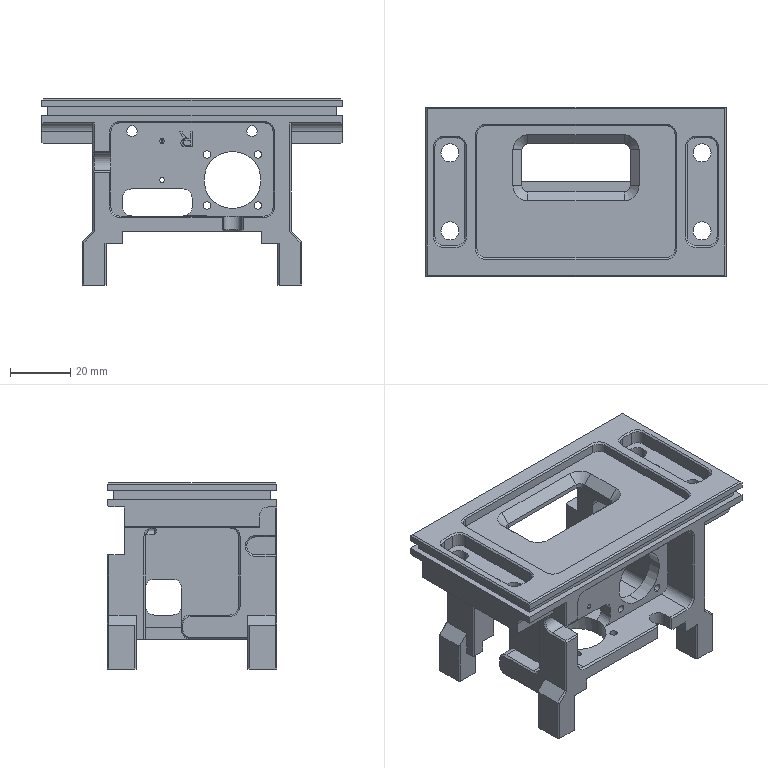CAM job | Mastercam | 3-axis milling, drilling | part box 100 x 56.5 x 62 mm | stock box 110 x 56.5 x 80 mm
Tools:
tool_number,name,type,diameter_mm,corner_radius_mm,flutes,flute_length_mm,overall_length_mm,shoulder_length_mm,holder_diameter_mm,length_offset,diameter_offset,default_rpm,default_feed_mm_min,default_plunge_mm_min,coolant
2,2 Flat End Mill,end mill,2,0,4,25,75,25,50,2,2,5000,600,600,COOL_OFF
2,2 Flat End Mill,end mill,2,0,4,25,75,25,50,2,2,5000,600,600,COOL_OFF
3,3 Flat End Mill,end mill,3,0,4,25,75,25,50,3,3,3333,399.96,600,COOL_OFF
3,3 Flat End Mill,end mill,3,0,4,25,75,25,50,3,3,3333,399.96,600,COOL_OFF
4,4 Flat End Mill,end mill,4,0,4,25,75,25,50,4,4,2500,300,600,COOL_OFF
4,4 Flat End Mill,end mill,4,0,4,25,75,25,50,4,4,2500,300,600,COOL_OFF
5,4 Chamfer Mill,chamfer mill,4,0,4,25,75,30,50,5,5,6250,750,600,COOL_OFF
5,4 Chamfer Mill,chamfer mill,4,0,4,25,75,30,50,5,5,6250,750,600,COOL_OFF
5,6 Flat End Mill,end mill,6,0,4,25,75,25,50,5,5,1667,200.04,600,COOL_OFF
6,6 Flat End Mill,end mill,6,0,4,25,75,25,50,6,6,1667,200.04,600,COOL_OFF
6,6 Flat End Mill,end mill,6,0,4,25,75,25,50,6,6,1667,200.04,600,COOL_OFF
11,12 Flat End Mill,end mill,12,0,4,25,75,25,50,11,11,8000,4000,600,COOL_OFF
11,12 Flat End Mill,end mill,12,0,4,25,75,25,50,11,11,8000,4000,600,COOL_OFF
12,12 Flat End Mill,end mill,12,0,4,25,75,25,50,12,12,833,99.96,600,COOL_OFF
12,12 Flat End Mill,end mill,12,0,4,25,75,25,50,12,12,833,99.96,600,COOL_OFF
13,16 Flat End Mill,end mill,16,0,4,25,75,25,50,13,13,5000,3000,600,COOL_OFF
13,Copy 16 Flat End Mill,end mill,16,0,4,25,75,25,50,13,13,5000,3000,600,COOL_OFF
13,16 Flat End Mill,end mill,16,0,4,25,75,25,50,13,13,5000,3000,600,COOL_OFF
14,6 Flat End Mill,end mill,6,0,4,25,75,25,50,14,14,5000,2000,600,COOL_OFF
14,Copy 6 Flat End Mill,end mill,6,0,4,25,75,25,50,14,14,5000,2000,600,COOL_OFF
15,4 Flat End Mill,end mill,4,0,4,25,75,25,50,15,15,6500,2000,600,COOL_OFF
15,Copy 4 Flat End Mill,end mill,4,0,4,25,75,25,50,15,15,6500,2000,600,COOL_OFF
16,16 Flat End Mill,end mill,16,0,4,25,75,25,50,16,16,625,75,600,COOL_OFF
16,16 Flat End Mill,end mill,16,0,4,25,75,25,50,16,16,5000,1000,600,COOL_OFF
17,14 Chamfer Mill,chamfer mill,14,0,4,25,75,30,50,17,17,1786,214.32,600,COOL_OFF
17,14 Chamfer Mill,chamfer mill,14,0,4,25,75,30,50,17,17,1786,214.32,600,COOL_OFF
18,6 Flat End Mill,end mill,6,0,4,25,75,25,50,18,18,1667,200.04,600,COOL_OFF
18,Copy 6 Flat End Mill,end mill,6,0,4,25,75,25,50,18,18,1667,200.04,600,COOL_OFF
20,63 Flat End Mill,end mill,63,0,4,25,75,25,50,20,20,4000,1000,600,COOL_OFF
20,63 Flat End Mill,end mill,63,0,4,25,75,25,50,20,20,159,19.08,600,COOL_OFF
Operations:
seq,operation,operation_type,tool_number,tool_name,tool_diameter_mm,spindle_rpm,feed_mm_min,plunge_mm_min,retract_mm_min,cycle_time_s,wcs,posted,nc_file
1,Facing - [WCS: Plane] - [Tplane: Plane],Facing,20,63 Flat End Mill,63,4000,1000,600,1200,24.268,Plane,yes,1.nc
2,2D High Speed (2D Dynamic Mill) - [WCS: Plane] - [Tplane: Plane],HighSpeed2D,13,16 Flat End Mill,16,5500,3000,600,1200,372.445,Plane,yes,1.nc
3,Contour (Ramp) - [WCS: Plane] - [Tplane: Plane],Contour,13,16 Flat End Mill,16,5500,1500,600,1200,67.168,Plane,yes,1.nc
4,Contour (2D) - [WCS: Plane] - [Tplane: Plane],Contour,16,16 Flat End Mill,16,5500,1000,600,1200,51.918,Plane,yes,1.nc
5,Contour (Remachining) - [WCS: Plane] - [Tplane: Plane],Contour,6,6 Flat End Mill,6,7000,3000,600,1200,34.787,Plane,yes,1.nc
6,Contour (2D) - [WCS: Plane] - [Tplane: Plane],Contour,6,6 Flat End Mill,6,7000,1000,600,1200,37.219,Plane,yes,1.nc
7,2D High Speed (2D Area Mill) - [WCS: Plane] - [Tplane: Plane],HighSpeed2D,6,6 Flat End Mill,6,7000,1000,600,1200,26.955,Plane,yes,1.nc
8,Contour (Ramp) - [WCS: Plane] - [Tplane: Plane],Contour,6,6 Flat End Mill,6,7000,1500,600,1200,26.435,Plane,yes,1.nc
9,Contour (2D) - [WCS: Plane] - [Tplane: Plane],Contour,6,6 Flat End Mill,6,7000,1000,600,1200,8.281,Plane,yes,1.nc
10,Contour (Ramp) - [WCS: Plane] - [Tplane: Plane],Contour,6,6 Flat End Mill,6,7000,1500,600,1200,17.872,Plane,yes,1.nc
11,Contour (2D) - [WCS: Plane] - [Tplane: Plane],Contour,6,6 Flat End Mill,6,7000,1000,600,1200,8.664,Plane,yes,1.nc
12,Contour (Ramp) - [WCS: Plane] - [Tplane: Plane],Contour,2,2 Flat End Mill,2,7000,3000,600,1200,42.583,Plane,yes,1.nc
13,Contour (2D) - [WCS: Plane] - [Tplane: Plane],Contour,2,2 Flat End Mill,2,7000,800,600,1200,16.213,Plane,yes,1.nc
14,Contour (2D chamfer) - [WCS: Plane] - [Tplane: Plane],Contour,5,6 Flat End Mill,6,7000,1200,600,1200,16.866,Plane,yes,1.nc
15,Contour (2D chamfer) - [WCS: Plane] - [Tplane: Plane],Contour,5,6 Flat End Mill,6,7000,1200,600,1200,8.527,Plane,yes,1.nc
16,Contour (2D chamfer) - [WCS: Plane] - [Tplane: Plane],Contour,5,6 Flat End Mill,6,7000,1200,600,1200,18.288,Plane,yes,1.nc
17,Drill/Counterbore - [WCS: Plane] - [Tplane: Plane],Drill,5,6 Flat End Mill,6,6500,200,600,1200,6.526,Plane,yes,1.nc
18,Facing - [WCS: Plane-1] - [Tplane: Plane-1],Facing,20,63 Flat End Mill,63,4000,2000,600,1200,235.558,Plane-1,yes,1.nc
19,Contour (Ramp) - [WCS: Plane-1] - [Tplane: Plane-1],Contour,11,12 Flat End Mill,12,8000,4000,600,1200,34.159,Plane-1,yes,1.nc
20,Contour (2D) - [WCS: Plane-1] - [Tplane: Plane-1],Contour,12,12 Flat End Mill,12,8000,1000,600,1200,15.085,Plane-1,yes,1.nc
21,2D High Speed (2D Area Mill) - [WCS: Plane-1] - [Tplane: Plane-1],HighSpeed2D,11,12 Flat End Mill,12,8000,4000,600,1200,192.884,Plane-1,yes,1.nc
22,Contour (2D) - [WCS: Plane-1] - [Tplane: Plane-1],Contour,12,12 Flat End Mill,12,8000,1000,600,1200,18.911,Plane-1,yes,1.nc
23,Contour (Ramp) - [WCS: Plane-1] - [Tplane: Plane-1],Contour,11,12 Flat End Mill,12,8000,2000,600,1200,44.183,Plane-1,yes,1.nc
24,Contour (2D) - [WCS: Plane-1] - [Tplane: Plane-1],Contour,12,12 Flat End Mill,12,8000,1000,600,1200,7.27,Plane-1,yes,1.nc
25,Contour (Ramp) - [WCS: Plane-1] - [Tplane: Plane-1],Contour,11,12 Flat End Mill,12,8000,2000,600,1200,42.433,Plane-1,yes,1.nc
26,Contour (Remachining) - [WCS: Plane-1] - [Tplane: Plane-1],Contour,14,Copy 6 Flat End Mill,6,5000,3000,600,1200,35.027,Plane-1,yes,1.nc
27,2D High Speed (2D Area Mill) - [WCS: Plane-1] - [Tplane: Plane-1],HighSpeed2D,14,Copy 6 Flat End Mill,6,5000,800,600,1200,32.203,Plane-1,yes,1.nc
28,Contour (2D) - [WCS: Plane-1] - [Tplane: Plane-1],Contour,14,Copy 6 Flat End Mill,6,5000,800,600,1200,37.956,Plane-1,yes,1.nc
29,Contour (Remachining) - [WCS: Plane-1] - [Tplane: Plane-1],Contour,15,Copy 4 Flat End Mill,4,5500,2000,600,1200,46.379,Plane-1,yes,1.nc
30,Contour (Remachining) - [WCS: Plane-1] - [Tplane: Plane-1],Contour,15,Copy 4 Flat End Mill,4,5500,800,600,1200,20.427,Plane-1,yes,1.nc
31,Contour (Ramp) - [WCS: Plane-1] - [Tplane: Plane-1],Contour,2,2 Flat End Mill,2,6500,2000,600,1200,94.193,Plane-1,yes,1.nc
32,Contour (2D) - [WCS: Plane-1] - [Tplane: Plane-1],Contour,2,2 Flat End Mill,2,6500,1000,600,1200,13.093,Plane-1,yes,1.nc
33,Drill/Counterbore - [WCS: Plane-1] - [Tplane: Plane-1],Drill,5,6 Flat End Mill,6,6500,200,600,1200,1.512,Plane-1,yes,1.nc
34,Contour (2D chamfer) - [WCS: Plane-1] - [Tplane: Plane-1],Contour,5,6 Flat End Mill,6,6500,1000,600,1200,6.992,Plane-1,yes,1.nc
35,Contour (2D chamfer) - [WCS: Plane-1] - [Tplane: Plane-1],Contour,5,6 Flat End Mill,6,6500,1000,600,1200,6.846,Plane-1,yes,1.nc
36,Contour (2D chamfer) - [WCS: Plane-1] - [Tplane: Plane-1],Contour,5,6 Flat End Mill,6,6500,1000,600,1200,10.432,Plane-1,yes,1.nc
37,Contour (2D chamfer) - [WCS: Plane-1] - [Tplane: Plane-1],Contour,5,6 Flat End Mill,6,6500,1000,600,1200,11.317,Plane-1,yes,1.nc
38,Contour (2D chamfer) - [WCS: Plane-1] - [Tplane: Plane-1],Contour,5,6 Flat End Mill,6,6500,1000,600,1200,20.167,Plane-1,yes,1.nc
39,2D High Speed (2D Area Mill) - [WCS: Plane-2] - [Tplane: Plane-2],HighSpeed2D,11,12 Flat End Mill,12,8000,4000,600,1200,39.518,Plane-2,yes,1.nc
40,Contour (Ramp) - [WCS: Plane-2] - [Tplane: Plane-2],Contour,11,12 Flat End Mill,12,8000,2000,600,1200,14.081,Plane-2,yes,1.nc
41,Contour (Ramp) - [WCS: Plane-2] - [Tplane: Plane-2],Contour,6,6 Flat End Mill,6,6500,3000,600,1200,36.258,Plane-2,yes,1.nc
42,Contour (2D) - [WCS: Plane-2] - [Tplane: Plane-2],Contour,6,6 Flat End Mill,6,6500,1000,600,1200,26.145,Plane-2,yes,1.nc
43,Contour (Remachining) - [WCS: Plane-2] - [Tplane: Plane-2],Contour,6,6 Flat End Mill,6,6500,3000,600,1200,8.854,Plane-2,yes,1.nc
44,2D High Speed (2D Area Mill) - [WCS: Plane-2] - [Tplane: Plane-2],HighSpeed2D,6,6 Flat End Mill,6,6500,1000,600,1200,68.692,Plane-2,yes,1.nc
45,Contour (2D) - [WCS: Plane-2] - [Tplane: Plane-2],Contour,6,6 Flat End Mill,6,6500,1000,600,1200,36.067,Plane-2,yes,1.nc
46,Contour (Remachining) - [WCS: Plane-2] - [Tplane: Plane-2],Contour,3,3 Flat End Mill,3,6500,2000,600,1200,29.382,Plane-2,yes,1.nc
47,Contour (2D) - [WCS: Plane-2] - [Tplane: Plane-2],Contour,3,3 Flat End Mill,3,6500,1000,600,1200,11.957,Plane-2,yes,1.nc
48,Drill/Counterbore - [WCS: Plane-2] - [Tplane: Plane-2],Drill,5,6 Flat End Mill,6,6500,200,600,1200,2.994,Plane-2,yes,1.nc
49,Contour (2D chamfer) - [WCS: Plane-2] - [Tplane: Plane-2],Contour,5,6 Flat End Mill,6,6500,1000,600,1200,43.634,Plane-2,yes,1.nc
50,Contour (2D chamfer) - [WCS: Plane-2] - [Tplane: Plane-2],Contour,17,14 Chamfer Mill,14,6500,1000,600,1200,26.895,Plane-2,yes,1.nc
51,Contour (Ramp) - [WCS: Plane-2] - [Tplane: Plane-2],Contour,4,4 Flat End Mill,4,7000,2000,600,1200,13.401,Plane-2,yes,1.nc
52,Contour (Ramp) - [WCS: Plane-2] - [Tplane: Plane-2],Contour,4,4 Flat End Mill,4,7000,500,600,1200,10.581,Plane-2,yes,1.nc
53,Contour (2D) - [WCS: Plane-3] - [Tplane: Plane-3],Contour,13,16 Flat End Mill,16,5500,3000,600,1200,145.31,Plane-3,yes,1.nc
54,Contour (Ramp) - [WCS: Plane-3] - [Tplane: Plane-3],Contour,13,16 Flat End Mill,16,5500,3000,600,1200,16.646,Plane-3,yes,1.nc
55,Contour (Ramp) - [WCS: Plane-3] - [Tplane: Plane-3],Contour,13,16 Flat End Mill,16,5500,3000,600,1200,18.755,Plane-3,yes,1.nc
56,Contour (Ramp) - [WCS: Plane-3] - [Tplane: Plane-3],Contour,13,16 Flat End Mill,16,5500,2000,600,1200,13.738,Plane-3,yes,1.nc
57,Facing - [WCS: Plane-3] - [Tplane: Plane-3],Facing,16,16 Flat End Mill,16,5500,1000,600,1200,4.49,Plane-3,yes,1.nc
58,Contour (2D) - [WCS: Plane-3] - [Tplane: Plane-3],Contour,16,16 Flat End Mill,16,5500,1000,600,1200,9.961,Plane-3,yes,1.nc
59,Contour (2D) - [WCS: Plane-3] - [Tplane: Plane-3],Contour,16,16 Flat End Mill,16,5500,1000,600,1200,11.19,Plane-3,yes,1.nc
60,Contour (Ramp) - [WCS: Plane-3] - [Tplane: Plane-3],Contour,6,6 Flat End Mill,6,6500,3000,600,1200,15.861,Plane-3,yes,1.nc
61,Contour (2D) - [WCS: Plane-3] - [Tplane: Plane-3],Contour,6,6 Flat End Mill,6,6500,1000,600,1200,6.801,Plane-3,yes,1.nc
62,Contour (Remachining) - [WCS: Plane-3] - [Tplane: Plane-3],Contour,6,6 Flat End Mill,6,6500,3000,600,1200,15.343,Plane-3,yes,1.nc
63,Contour (2D) - [WCS: Plane-3] - [Tplane: Plane-3],Contour,6,6 Flat End Mill,6,6500,1000,600,1200,6.417,Plane-3,yes,1.nc
64,2D High Speed (2D Area Mill) - [WCS: Plane-3] - [Tplane: Plane-3],HighSpeed2D,6,6 Flat End Mill,6,6500,1000,600,1200,20.992,Plane-3,yes,1.nc
65,Contour (Ramp) - [WCS: Plane-3] - [Tplane: Plane-3],Contour,6,6 Flat End Mill,6,6500,2000,600,1200,30.854,Plane-3,yes,1.nc
66,Contour (2D) - [WCS: Plane-3] - [Tplane: Plane-3],Contour,6,6 Flat End Mill,6,6500,1000,600,1200,4.121,Plane-3,yes,1.nc
67,Contour (2D chamfer) - [WCS: Plane-3] - [Tplane: Plane-3],Contour,17,14 Chamfer Mill,14,6500,1000,600,1200,21.117,Plane-3,yes,1.nc
68,Contour (Ramp) - [WCS: Plane-3] - [Tplane: Plane-3],Contour,2,2 Flat End Mill,2,6500,3000,600,1200,32.443,Plane-3,yes,1.nc
69,Contour (2D) - [WCS: Plane-3] - [Tplane: Plane-3],Contour,2,2 Flat End Mill,2,6500,1000,600,1200,7.873,Plane-3,yes,1.nc
70,Contour (2D chamfer) - [WCS: Plane-3] - [Tplane: Plane-3],Contour,5,6 Flat End Mill,6,6500,1000,600,1200,3.572,Plane-3,yes,1.nc
71,Contour (2D chamfer) - [WCS: Plane-3] - [Tplane: Plane-3],Contour,5,6 Flat End Mill,6,6500,1000,600,1200,5.258,Plane-3,yes,1.nc
72,Contour (2D chamfer) - [WCS: Plane-3] - [Tplane: Plane-3],Contour,5,6 Flat End Mill,6,6500,1000,600,1200,9.836,Plane-3,yes,1.nc
73,Contour (Ramp) - [WCS: Plane-10] - [Tplane: Plane-10],Contour,13,16 Flat End Mill,16,5500,3000,600,1200,127.451,Plane-10,yes,1.nc
74,Contour (Ramp) - [WCS: Plane-10] - [Tplane: Plane-10],Contour,13,16 Flat End Mill,16,5500,3000,600,1200,16.665,Plane-10,yes,1.nc
75,Contour (Ramp) - [WCS: Plane-10] - [Tplane: Plane-10],Contour,13,16 Flat End Mill,16,5500,3000,600,1200,18.755,Plane-10,yes,1.nc
76,Facing - [WCS: Plane-10] - [Tplane: Plane-10],Facing,16,16 Flat End Mill,16,5500,1000,600,1200,4.49,Plane-10,yes,1.nc
77,Contour (2D) - [WCS: Plane-10] - [Tplane: Plane-10],Contour,16,16 Flat End Mill,16,5500,1000,600,1200,10.441,Plane-10,yes,1.nc
78,Contour (2D) - [WCS: Plane-10] - [Tplane: Plane-10],Contour,16,16 Flat End Mill,16,5500,1000,600,1200,11.19,Plane-10,yes,1.nc
79,2D High Speed (2D Area Mill) - [WCS: Plane-10] - [Tplane: Plane-10],HighSpeed2D,6,6 Flat End Mill,6,6500,3000,600,1200,94.317,Plane-10,yes,1.nc
80,2D High Speed (2D Area Mill) - [WCS: Plane-10] - [Tplane: Plane-10],HighSpeed2D,6,6 Flat End Mill,6,6500,1000,600,1200,27.332,Plane-10,yes,1.nc
81,Contour (2D) - [WCS: Plane-10] - [Tplane: Plane-10],Contour,6,6 Flat End Mill,6,6500,1000,600,1200,8.748,Plane-10,yes,1.nc
82,Contour (Ramp) - [WCS: Plane-10] - [Tplane: Plane-10],Contour,6,6 Flat End Mill,6,6500,1500,600,1200,29.271,Plane-10,yes,1.nc
83,Contour (2D) - [WCS: Plane-10] - [Tplane: Plane-10],Contour,6,6 Flat End Mill,6,6500,800,600,1200,4.795,Plane-10,yes,1.nc
84,Contour (Ramp) - [WCS: Plane-10] - [Tplane: Plane-10],Contour,6,6 Flat End Mill,6,6500,3000,600,1200,15.861,Plane-10,yes,1.nc
85,Contour (2D) - [WCS: Plane-10] - [Tplane: Plane-10],Contour,6,6 Flat End Mill,6,6500,1000,600,1200,6.801,Plane-10,yes,1.nc
86,Contour (Ramp) - [WCS: Plane-10] - [Tplane: Plane-10],Contour,4,4 Flat End Mill,4,5000,2000,600,1200,21.87,Plane-10,yes,1.nc
87,Contour (2D) - [WCS: Plane-10] - [Tplane: Plane-10],Contour,4,4 Flat End Mill,4,5000,800,600,1200,7.806,Plane-10,yes,1.nc
88,Contour (Ramp) - [WCS: Plane-10] - [Tplane: Plane-10],Contour,2,2 Flat End Mill,2,6500,3000,600,1200,25.183,Plane-10,yes,1.nc
89,Contour (2D) - [WCS: Plane-10] - [Tplane: Plane-10],Contour,2,2 Flat End Mill,2,6500,800,600,1200,9.688,Plane-10,yes,1.nc
90,Contour (2D chamfer) - [WCS: Plane-10] - [Tplane: Plane-10],Contour,5,6 Flat End Mill,6,6000,1000,600,1200,13.085,Plane-10,yes,1.nc
91,Contour (2D chamfer) - [WCS: Plane-10] - [Tplane: Plane-10],Contour,5,6 Flat End Mill,6,6000,1000,600,1200,6.34,Plane-10,yes,1.nc
92,Contour (2D chamfer) - [WCS: Plane-10] - [Tplane: Plane-10],Contour,5,6 Flat End Mill,6,6500,1000,600,1200,2.284,Plane-10,yes,1.nc
93,Contour (2D chamfer) - [WCS: Plane-10] - [Tplane: Plane-10],Contour,17,14 Chamfer Mill,14,6500,1000,600,1200,22.707,Plane-10,yes,1.nc
94,Contour (Ramp) - [WCS: Plane-11] - [Tplane: Plane-11],Contour,11,12 Flat End Mill,12,8000,4000,600,1200,185.263,Plane-11,yes,1.nc
95,Contour (Ramp) - [WCS: Plane-11] - [Tplane: Plane-11],Contour,11,12 Flat End Mill,12,8000,4000,600,1200,30.268,Plane-11,yes,1.nc
96,Contour (2D) - [WCS: Plane-11] - [Tplane: Plane-11],Contour,12,12 Flat End Mill,12,8000,1000,600,1200,9.423,Plane-11,yes,1.nc
97,Contour (2D) - [WCS: Plane-11] - [Tplane: Plane-11],Contour,12,12 Flat End Mill,12,8000,1000,600,1200,29.636,Plane-11,yes,1.nc
98,Contour (Ramp) - [WCS: Plane-11] - [Tplane: Plane-11],Contour,11,12 Flat End Mill,12,8000,4000,600,1200,53.666,Plane-11,yes,1.nc
99,Contour (2D) - [WCS: Plane-11] - [Tplane: Plane-11],Contour,12,12 Flat End Mill,12,8000,1000,600,1200,14.427,Plane-11,yes,1.nc
100,Contour (Ramp) - [WCS: Plane-11] - [Tplane: Plane-11],Contour,6,6 Flat End Mill,6,6500,2000,600,1200,28.852,Plane-11,yes,1.nc
101,Contour (2D) - [WCS: Plane-11] - [Tplane: Plane-11],Contour,6,6 Flat End Mill,6,6500,1000,600,1200,8.348,Plane-11,yes,1.nc
102,Contour (Ramp) - [WCS: Plane-11] - [Tplane: Plane-11],Contour,4,4 Flat End Mill,4,5000,2000,600,1200,13.304,Plane-11,yes,1.nc
103,Contour (2D) - [WCS: Plane-11] - [Tplane: Plane-11],Contour,4,4 Flat End Mill,4,5000,800,600,1200,4.177,Plane-11,yes,1.nc
104,Contour (Ramp) - [WCS: Plane-11] - [Tplane: Plane-11],Contour,18,Copy 6 Flat End Mill,6,4500,800,600,1200,542.698,Plane-11,yes,1.nc
105,Drill/Counterbore - [WCS: Plane-11] - [Tplane: Plane-11],Drill,5,6 Flat End Mill,6,6000,200,600,1200,7.169,Plane-11,yes,1.nc
106,Contour (2D chamfer) - [WCS: Plane-11] - [Tplane: Plane-11],Contour,5,6 Flat End Mill,6,6000,1000,600,1200,1.46,Plane-11,yes,1.nc
107,Contour (2D chamfer) - [WCS: Plane-11] - [Tplane: Plane-11],Contour,5,6 Flat End Mill,6,6000,1000,600,1200,1.814,Plane-11,yes,1.nc
108,Contour (2D chamfer) - [WCS: Plane-11] - [Tplane: Plane-11],Contour,5,6 Flat End Mill,6,6000,1000,600,1200,30.44,Plane-11,yes,1.nc
109,Facing - [WCS: Plane-4] - [Tplane: Plane-4],Facing,20,63 Flat End Mill,63,4000,1000,600,1200,25.273,Plane-4,yes,2.nc
110,2D High Speed (2D Dynamic Mill) - [WCS: Plane-4] - [Tplane: Plane-4],HighSpeed2D,13,16 Flat End Mill,16,5500,3000,600,1200,376.909,Plane-4,yes,2.nc
111,Contour (Ramp) - [WCS: Plane-4] - [Tplane: Plane-4],Contour,13,16 Flat End Mill,16,5500,2000,600,1200,78.629,Plane-4,yes,2.nc
112,Contour (2D) - [WCS: Plane-4] - [Tplane: Plane-4],Contour,16,16 Flat End Mill,16,5000,1000,600,1200,104.157,Plane-4,yes,2.nc
113,Contour (Remachining) - [WCS: Plane-4] - [Tplane: Plane-4],Contour,6,6 Flat End Mill,6,6500,3000,600,1200,34.798,Plane-4,yes,2.nc
114,2D High Speed (2D Area Mill) - [WCS: Plane-4] - [Tplane: Plane-4],HighSpeed2D,6,6 Flat End Mill,6,6500,1000,600,1200,38.478,Plane-4,yes,2.nc
115,Contour (2D) - [WCS: Plane-4] - [Tplane: Plane-4],Contour,6,6 Flat End Mill,6,6500,1000,600,1200,55.037,Plane-4,yes,2.nc
116,Contour (Ramp) - [WCS: Plane-4] - [Tplane: Plane-4],Contour,6,6 Flat End Mill,6,6500,1500,600,1200,26.435,Plane-4,yes,2.nc
117,Contour (2D) - [WCS: Plane-4] - [Tplane: Plane-4],Contour,6,6 Flat End Mill,6,6500,1000,600,1200,8.281,Plane-4,yes,2.nc
118,Contour (Ramp) - [WCS: Plane-4] - [Tplane: Plane-4],Contour,6,6 Flat End Mill,6,6500,1500,600,1200,17.872,Plane-4,yes,2.nc
119,Contour (2D) - [WCS: Plane-4] - [Tplane: Plane-4],Contour,6,6 Flat End Mill,6,6500,1000,600,1200,8.188,Plane-4,yes,2.nc
120,Contour (Ramp) - [WCS: Plane-4] - [Tplane: Plane-4],Contour,2,2 Flat End Mill,2,10000,2500,600,1200,50.903,Plane-4,yes,2.nc
121,Contour (2D) - [WCS: Plane-4] - [Tplane: Plane-4],Contour,2,2 Flat End Mill,2,6500,800,600,1200,16.213,Plane-4,yes,2.nc
122,Contour (2D) - [WCS: Plane-4] - [Tplane: Plane-4],Contour,16,16 Flat End Mill,16,5000,1000,600,1200,104.157,Plane-4,yes,2.nc
123,Contour (2D chamfer) - [WCS: Plane-4] - [Tplane: Plane-4],Contour,5,6 Flat End Mill,6,6500,1000,600,1200,41.201,Plane-4,yes,2.nc
124,Contour (2D chamfer) - [WCS: Plane-4] - [Tplane: Plane-4],Contour,5,6 Flat End Mill,6,6500,1000,600,1200,10.154,Plane-4,yes,2.nc
125,Drill/Counterbore - [WCS: Plane-4] - [Tplane: Plane-4],Drill,5,6 Flat End Mill,6,6000,200,600,1200,6.526,Plane-4,yes,2.nc
126,Facing - [WCS: Plane-5] - [Tplane: Plane-5],Facing,20,63 Flat End Mill,63,4000,2000,600,1200,225.995,Plane-5,yes,2.nc
127,Contour (Ramp) - [WCS: Plane-5] - [Tplane: Plane-5],Contour,11,12 Flat End Mill,12,8000,4000,600,1200,32.539,Plane-5,yes,2.nc
128,Contour (2D) - [WCS: Plane-5] - [Tplane: Plane-5],Contour,12,12 Flat End Mill,12,8000,1000,600,1200,14.365,Plane-5,yes,2.nc
129,2D High Speed (2D Area Mill) - [WCS: Plane-5] - [Tplane: Plane-5],HighSpeed2D,11,12 Flat End Mill,12,8000,4000,600,1200,192.884,Plane-5,yes,2.nc
130,Contour (2D) - [WCS: Plane-5] - [Tplane: Plane-5],Contour,12,12 Flat End Mill,12,8000,1000,600,1200,18.911,Plane-5,yes,2.nc
131,Contour (Ramp) - [WCS: Plane-5] - [Tplane: Plane-5],Contour,11,12 Flat End Mill,12,8000,2000,600,1200,44.183,Plane-5,yes,2.nc
132,Contour (2D) - [WCS: Plane-5] - [Tplane: Plane-5],Contour,12,12 Flat End Mill,12,8000,1000,600,1200,7.27,Plane-5,yes,2.nc
133,Contour (Ramp) - [WCS: Plane-5] - [Tplane: Plane-5],Contour,11,12 Flat End Mill,12,8000,2000,600,1200,42.433,Plane-5,yes,2.nc
134,Contour (Remachining) - [WCS: Plane-5] - [Tplane: Plane-5],Contour,14,Copy 6 Flat End Mill,6,5000,2000,600,1200,74.663,Plane-5,yes,2.nc
135,2D High Speed (2D Area Mill) - [WCS: Plane-5] - [Tplane: Plane-5],HighSpeed2D,14,Copy 6 Flat End Mill,6,5000,800,600,1200,23.179,Plane-5,yes,2.nc
136,Contour (2D) - [WCS: Plane-5] - [Tplane: Plane-5],Contour,14,Copy 6 Flat End Mill,6,5000,800,600,1200,37.956,Plane-5,yes,2.nc
137,Contour (Remachining) - [WCS: Plane-5] - [Tplane: Plane-5],Contour,15,Copy 4 Flat End Mill,4,5000,1500,600,1200,75.53,Plane-5,yes,2.nc
138,Contour (Remachining) - [WCS: Plane-5] - [Tplane: Plane-5],Contour,15,Copy 4 Flat End Mill,4,5000,800,600,1200,20.427,Plane-5,yes,2.nc
139,Contour (Ramp) - [WCS: Plane-5] - [Tplane: Plane-5],Contour,2,2 Flat End Mill,2,6500,3000,600,1200,42.583,Plane-5,yes,2.nc
140,Contour (2D) - [WCS: Plane-5] - [Tplane: Plane-5],Contour,2,2 Flat End Mill,2,6500,1000,600,1200,13.093,Plane-5,yes,2.nc
141,Drill/Counterbore - [WCS: Plane-5] - [Tplane: Plane-5],Drill,5,6 Flat End Mill,6,6000,200,600,1200,1.512,Plane-5,yes,2.nc
142,Contour (2D chamfer) - [WCS: Plane-5] - [Tplane: Plane-5],Contour,5,6 Flat End Mill,6,6000,1000,600,1200,6.846,Plane-5,yes,2.nc
143,Contour (2D chamfer) - [WCS: Plane-5] - [Tplane: Plane-5],Contour,5,6 Flat End Mill,6,6000,1000,600,1200,54.417,Plane-5,yes,2.nc
144,Contour (2D chamfer) - [WCS: Plane-5] - [Tplane: Plane-5],Contour,5,6 Flat End Mill,6,6000,1000,600,1200,6.872,Plane-5,yes,2.nc
145,2D High Speed (2D Area Mill) - [WCS: Plane-6] - [Tplane: Plane-6],HighSpeed2D,12,12 Flat End Mill,12,8000,4000,600,1200,38.257,Plane-6,yes,2.nc
146,Contour (Ramp) - [WCS: Plane-6] - [Tplane: Plane-6],Contour,12,12 Flat End Mill,12,8000,2000,600,1200,14.081,Plane-6,yes,2.nc
147,Contour (Remachining) - [WCS: Plane-6] - [Tplane: Plane-6],Contour,6,6 Flat End Mill,6,6500,3000,600,1200,8.987,Plane-6,yes,2.nc
148,2D High Speed (2D Area Mill) - [WCS: Plane-6] - [Tplane: Plane-6],HighSpeed2D,6,6 Flat End Mill,6,6500,1000,600,1200,68.264,Plane-6,yes,2.nc
149,Contour (2D) - [WCS: Plane-6] - [Tplane: Plane-6],Contour,6,6 Flat End Mill,6,6500,1000,600,1200,36.067,Plane-6,yes,2.nc
150,Contour (Ramp) - [WCS: Plane-6] - [Tplane: Plane-6],Contour,6,6 Flat End Mill,6,6500,2000,600,1200,61.132,Plane-6,yes,2.nc
151,Contour (2D) - [WCS: Plane-6] - [Tplane: Plane-6],Contour,6,6 Flat End Mill,6,6500,1000,600,1200,26.107,Plane-6,yes,2.nc
152,Contour (Remachining) - [WCS: Plane-6] - [Tplane: Plane-6],Contour,3,3 Flat End Mill,3,6500,3000,600,1200,18.222,Plane-6,yes,2.nc
153,Contour (Ramp) - [WCS: Plane-6] - [Tplane: Plane-6],Contour,3,3 Flat End Mill,3,6500,1000,600,1200,15.033,Plane-6,yes,2.nc
154,Drill/Counterbore - [WCS: Plane-6] - [Tplane: Plane-6],Drill,5,6 Flat End Mill,6,6000,200,600,1200,2.994,Plane-6,yes,2.nc
155,Contour (2D chamfer) - [WCS: Plane-6] - [Tplane: Plane-6],Contour,5,6 Flat End Mill,6,6000,1000,600,1200,43.634,Plane-6,yes,2.nc
156,Contour (2D chamfer) - [WCS: Plane-6] - [Tplane: Plane-6],Contour,17,14 Chamfer Mill,14,6500,1500,600,1200,28.146,Plane-6,yes,2.nc
157,Contour (Ramp) - [WCS: Plane-6] - [Tplane: Plane-6],Contour,4,4 Flat End Mill,4,7000,2000,600,1200,13.326,Plane-6,yes,2.nc
158,Contour (Ramp) - [WCS: Plane-6] - [Tplane: Plane-6],Contour,4,4 Flat End Mill,4,7000,1000,600,1200,6.046,Plane-6,yes,2.nc
159,Contour (Ramp) - [WCS: Plane-7] - [Tplane: Plane-7],Contour,13,16 Flat End Mill,16,5500,3000,600,1200,127.465,Plane-7,yes,2.nc
160,Contour (Ramp) - [WCS: Plane-7] - [Tplane: Plane-7],Contour,13,16 Flat End Mill,16,5500,3000,600,1200,16.646,Plane-7,yes,2.nc
161,Contour (Ramp) - [WCS: Plane-7] - [Tplane: Plane-7],Contour,13,16 Flat End Mill,16,5500,3000,600,1200,18.755,Plane-7,yes,2.nc
162,Contour (Ramp) - [WCS: Plane-7] - [Tplane: Plane-7],Contour,13,16 Flat End Mill,16,5500,2000,600,1200,14.21,Plane-7,yes,2.nc
163,Facing - [WCS: Plane-7] - [Tplane: Plane-7],Facing,16,16 Flat End Mill,16,5500,1000,600,1200,4.49,Plane-7,yes,2.nc
164,Contour (2D) - [WCS: Plane-7] - [Tplane: Plane-7],Contour,16,16 Flat End Mill,16,5500,1000,600,1200,10.201,Plane-7,yes,2.nc
165,Contour (2D) - [WCS: Plane-7] - [Tplane: Plane-7],Contour,16,16 Flat End Mill,16,5500,1000,600,1200,11.19,Plane-7,yes,2.nc
166,Contour (Ramp) - [WCS: Plane-7] - [Tplane: Plane-7],Contour,6,6 Flat End Mill,6,6500,3000,600,1200,15.861,Plane-7,yes,2.nc
167,Contour (2D) - [WCS: Plane-7] - [Tplane: Plane-7],Contour,6,6 Flat End Mill,6,6500,1000,600,1200,6.801,Plane-7,yes,2.nc
168,Contour (Remachining) - [WCS: Plane-7] - [Tplane: Plane-7],Contour,6,6 Flat End Mill,6,6500,3000,600,1200,15.341,Plane-7,yes,2.nc
169,2D High Speed (2D Area Mill) - [WCS: Plane-7] - [Tplane: Plane-7],HighSpeed2D,6,6 Flat End Mill,6,6500,1000,600,1200,19.336,Plane-7,yes,2.nc
170,Contour (2D) - [WCS: Plane-7] - [Tplane: Plane-7],Contour,6,6 Flat End Mill,6,6500,1000,600,1200,6.417,Plane-7,yes,2.nc
171,Contour (Ramp) - [WCS: Plane-7] - [Tplane: Plane-7],Contour,6,6 Flat End Mill,6,6500,1500,600,1200,31.431,Plane-7,yes,2.nc
172,Contour (2D) - [WCS: Plane-7] - [Tplane: Plane-7],Contour,6,6 Flat End Mill,6,6500,800,600,1200,5.095,Plane-7,yes,2.nc
173,Contour (Ramp) - [WCS: Plane-7] - [Tplane: Plane-7],Contour,2,2 Flat End Mill,2,6500,3000,600,1200,25.183,Plane-7,yes,2.nc
174,Contour (2D) - [WCS: Plane-7] - [Tplane: Plane-7],Contour,2,2 Flat End Mill,2,6500,800,600,1200,9.688,Plane-7,yes,2.nc
175,Contour (2D chamfer) - [WCS: Plane-7] - [Tplane: Plane-7],Contour,17,14 Chamfer Mill,14,6500,1500,600,1200,19.145,Plane-7,yes,2.nc
176,Contour (2D chamfer) - [WCS: Plane-7] - [Tplane: Plane-7],Contour,5,6 Flat End Mill,6,6000,1000,600,1200,17.136,Plane-7,yes,2.nc
177,Contour (2D chamfer) - [WCS: Plane-7] - [Tplane: Plane-7],Contour,5,6 Flat End Mill,6,6000,1000,600,1200,20.711,Plane-7,yes,2.nc
178,Contour (Ramp) - [WCS: Plane-8] - [Tplane: Plane-8],Contour,13,16 Flat End Mill,16,5500,3000,600,1200,127.465,Plane-8,yes,2.nc
179,Contour (Ramp) - [WCS: Plane-8] - [Tplane: Plane-8],Contour,13,16 Flat End Mill,16,5500,3000,600,1200,16.646,Plane-8,yes,2.nc
180,Contour (Ramp) - [WCS: Plane-8] - [Tplane: Plane-8],Contour,13,16 Flat End Mill,16,5500,3000,600,1200,18.755,Plane-8,yes,2.nc
181,Facing - [WCS: Plane-8] - [Tplane: Plane-8],Facing,16,16 Flat End Mill,16,5500,1000,600,1200,4.49,Plane-8,yes,2.nc
182,Contour (2D) - [WCS: Plane-8] - [Tplane: Plane-8],Contour,16,16 Flat End Mill,16,5500,1000,600,1200,9.961,Plane-8,yes,2.nc
183,Contour (2D) - [WCS: Plane-8] - [Tplane: Plane-8],Contour,16,16 Flat End Mill,16,5500,1000,600,1200,11.19,Plane-8,yes,2.nc
184,Contour (Ramp) - [WCS: Plane-8] - [Tplane: Plane-8],Contour,6,6 Flat End Mill,6,6500,3000,600,1200,15.861,Plane-8,yes,2.nc
185,Contour (2D) - [WCS: Plane-8] - [Tplane: Plane-8],Contour,6,6 Flat End Mill,6,6500,1000,600,1200,6.801,Plane-8,yes,2.nc
186,2D High Speed (2D Area Mill) - [WCS: Plane-8] - [Tplane: Plane-8],HighSpeed2D,6,6 Flat End Mill,6,6500,3000,600,1200,93.844,Plane-8,yes,2.nc
187,2D High Speed (2D Area Mill) - [WCS: Plane-8] - [Tplane: Plane-8],HighSpeed2D,6,6 Flat End Mill,6,6500,1000,600,1200,27.639,Plane-8,yes,2.nc
188,Contour (2D) - [WCS: Plane-8] - [Tplane: Plane-8],Contour,6,6 Flat End Mill,6,6500,1000,600,1200,8.628,Plane-8,yes,2.nc
189,Contour (Ramp) - [WCS: Plane-8] - [Tplane: Plane-8],Contour,6,6 Flat End Mill,6,6500,1500,600,1200,28.739,Plane-8,yes,2.nc
190,Contour (2D) - [WCS: Plane-8] - [Tplane: Plane-8],Contour,6,6 Flat End Mill,6,6500,800,600,1200,4.795,Plane-8,yes,2.nc
191,Contour (Ramp) - [WCS: Plane-8] - [Tplane: Plane-8],Contour,4,4 Flat End Mill,4,5000,2000,600,1200,21.09,Plane-8,yes,2.nc
192,Contour (2D) - [WCS: Plane-8] - [Tplane: Plane-8],Contour,4,4 Flat End Mill,4,5000,800,600,1200,7.574,Plane-8,yes,2.nc
193,Contour (Ramp) - [WCS: Plane-8] - [Tplane: Plane-8],Contour,2,2 Flat End Mill,2,6500,3000,600,1200,25.183,Plane-8,yes,2.nc
194,Contour (2D) - [WCS: Plane-8] - [Tplane: Plane-8],Contour,2,2 Flat End Mill,2,6500,800,600,1200,9.688,Plane-8,yes,2.nc
195,Contour (2D chamfer) - [WCS: Plane-8] - [Tplane: Plane-8],Contour,5,6 Flat End Mill,6,6000,1000,600,1200,13.085,Plane-8,yes,2.nc
196,Contour (2D chamfer) - [WCS: Plane-8] - [Tplane: Plane-8],Contour,5,6 Flat End Mill,6,6000,1000,600,1200,23.411,Plane-8,yes,2.nc
197,Contour (2D chamfer) - [WCS: Plane-8] - [Tplane: Plane-8],Contour,5,6 Flat End Mill,6,6000,1000,600,1200,2.284,Plane-8,yes,2.nc
198,Contour (2D chamfer) - [WCS: Plane-8] - [Tplane: Plane-8],Contour,17,14 Chamfer Mill,14,6500,1000,600,1200,25.261,Plane-8,yes,2.nc
199,Contour (Ramp) - [WCS: Plane-9] - [Tplane: Plane-9],Contour,11,12 Flat End Mill,12,8000,3000,600,1200,191.472,Plane-9,yes,2.nc
200,Contour (Ramp) - [WCS: Plane-9] - [Tplane: Plane-9],Contour,11,12 Flat End Mill,12,8000,3000,600,1200,41.743,Plane-9,yes,2.nc
201,Contour (2D) - [WCS: Plane-9] - [Tplane: Plane-9],Contour,12,12 Flat End Mill,12,8000,1000,600,1200,31.153,Plane-9,yes,2.nc
202,Contour (2D) - [WCS: Plane-9] - [Tplane: Plane-9],Contour,12,12 Flat End Mill,12,8000,1000,600,1200,9.903,Plane-9,yes,2.nc
203,Contour (Ramp) - [WCS: Plane-9] - [Tplane: Plane-9],Contour,11,12 Flat End Mill,12,8000,3000,600,1200,77.668,Plane-9,yes,2.nc
204,Contour (2D) - [WCS: Plane-9] - [Tplane: Plane-9],Contour,12,12 Flat End Mill,12,8000,1000,600,1200,16.424,Plane-9,yes,2.nc
205,Contour (Ramp) - [WCS: Plane-9] - [Tplane: Plane-9],Contour,6,6 Flat End Mill,6,6500,2000,600,1200,23.603,Plane-9,yes,2.nc
206,Contour (2D) - [WCS: Plane-9] - [Tplane: Plane-9],Contour,6,6 Flat End Mill,6,6500,1000,600,1200,8.92,Plane-9,yes,2.nc
207,Contour (Ramp) - [WCS: Plane-9] - [Tplane: Plane-9],Contour,4,4 Flat End Mill,4,5000,2000,600,1200,16.65,Plane-9,yes,2.nc
208,Contour (2D) - [WCS: Plane-9] - [Tplane: Plane-9],Contour,4,4 Flat End Mill,4,5000,1000,600,1200,5.077,Plane-9,yes,2.nc
209,Contour (Ramp) - [WCS: Plane-9] - [Tplane: Plane-9],Contour,18,Copy 6 Flat End Mill,6,4500,1000,600,1200,292.867,Plane-9,yes,2.nc
210,Contour (2D chamfer) - [WCS: Plane-9] - [Tplane: Plane-9],Contour,5,6 Flat End Mill,6,6000,1000,600,1200,1.46,Plane-9,yes,2.nc
211,Contour (2D chamfer) - [WCS: Plane-9] - [Tplane: Plane-9],Contour,5,6 Flat End Mill,6,6000,1000,600,1200,1.694,Plane-9,yes,2.nc
212,Contour (2D chamfer) - [WCS: Plane-9] - [Tplane: Plane-9],Contour,5,6 Flat End Mill,6,6000,1000,600,1200,27.77,Plane-9,yes,2.nc
213,Drill/Counterbore - [WCS: Plane-9] - [Tplane: Plane-9],Drill,5,6 Flat End Mill,6,6000,200,600,1200,7.169,Plane-9,yes,2.nc